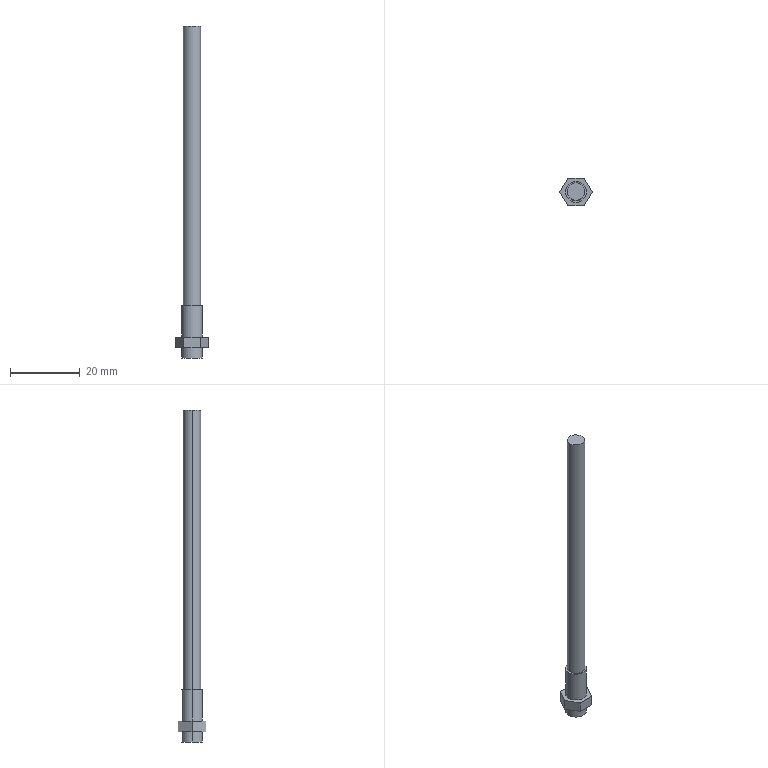Part | SolidWorks | features BaseBody 1 | 1 solid | 17 faces | box 9.238 x 8 x 95 mm | volume 2076 mm3 | plane 11 | cylinder 6 | commonest cylinder face diameters 6 x4 5 x2
STEP:
#1=CARTESIAN_POINT('',(-3.,0.,-15.));
#2=VERTEX_POINT('',#1);
#3=CARTESIAN_POINT('',(3.,0.,-15.));
#4=VERTEX_POINT('',#3);
#5=CARTESIAN_POINT('',(0.,0.,-15.));
#6=DIRECTION('',(0.,0.,-1.));
#7=DIRECTION('',(-1.,0.,0.));
#8=AXIS2_PLACEMENT_3D('',#5,#6,#7);
#9=CIRCLE('',#8,3.);
#10=EDGE_CURVE('',#2,#4,#9,.T.);
#11=ORIENTED_EDGE('',*,*,#10,.F.);
#12=CARTESIAN_POINT('',(-3.,0.,-12.));
#13=VERTEX_POINT('',#12);
#14=CARTESIAN_POINT('',(-3.,0.,-15.));
#15=DIRECTION('',(0.,0.,1.));
#16=VECTOR('',#15,1000.);
#17=LINE('',#14,#16);
#18=EDGE_CURVE('',#2,#13,#17,.T.);
#19=ORIENTED_EDGE('',*,*,#18,.T.);
#20=CARTESIAN_POINT('',(3.,0.,-12.));
#21=VERTEX_POINT('',#20);
#22=CARTESIAN_POINT('',(0.,0.,-12.));
#23=DIRECTION('',(0.,0.,-1.));
#24=DIRECTION('',(-1.,0.,0.));
#25=AXIS2_PLACEMENT_3D('',#22,#23,#24);
#26=CIRCLE('',#25,3.);
#27=EDGE_CURVE('',#13,#21,#26,.T.);
#28=ORIENTED_EDGE('',*,*,#27,.T.);
#29=CARTESIAN_POINT('',(3.,0.,-15.));
#30=DIRECTION('',(0.,0.,1.));
#31=VECTOR('',#30,1000.);
#32=LINE('',#29,#31);
#33=EDGE_CURVE('',#4,#21,#32,.T.);
#34=ORIENTED_EDGE('',*,*,#33,.F.);
#35=EDGE_LOOP('',(#11,#19,#28,#34));
#36=FACE_OUTER_BOUND('',#35,.T.);
#37=CARTESIAN_POINT('',(0.,0.,-15.));
#38=DIRECTION('',(0.,0.,1.));
#39=DIRECTION('',(1.,0.,0.));
#40=AXIS2_PLACEMENT_3D('',#37,#38,#39);
#41=CYLINDRICAL_SURFACE('',#40,3.);
#42=ADVANCED_FACE('',(#36),#41,.T.);
#43=CARTESIAN_POINT('',(2.5,0.,80.));
#44=VERTEX_POINT('',#43);
#45=CARTESIAN_POINT('',(-2.5,0.,80.));
#46=VERTEX_POINT('',#45);
#47=CARTESIAN_POINT('',(0.,0.,80.));
#48=DIRECTION('',(0.,0.,1.));
#49=DIRECTION('',(1.,0.,0.));
#50=AXIS2_PLACEMENT_3D('',#47,#48,#49);
#51=CIRCLE('',#50,2.5);
#52=EDGE_CURVE('',#44,#46,#51,.T.);
#53=ORIENTED_EDGE('',*,*,#52,.F.);
#54=CARTESIAN_POINT('',(2.5,0.,0.));
#55=VERTEX_POINT('',#54);
#56=CARTESIAN_POINT('',(2.5,0.,80.));
#57=DIRECTION('',(0.,0.,-1.));
#58=VECTOR('',#57,1000.);
#59=LINE('',#56,#58);
#60=EDGE_CURVE('',#44,#55,#59,.T.);
#61=ORIENTED_EDGE('',*,*,#60,.T.);
#62=CARTESIAN_POINT('',(-2.5,0.,0.));
#63=VERTEX_POINT('',#62);
#64=CARTESIAN_POINT('',(0.,0.,0.));
#65=DIRECTION('',(0.,0.,1.));
#66=DIRECTION('',(1.,0.,0.));
#67=AXIS2_PLACEMENT_3D('',#64,#65,#66);
#68=CIRCLE('',#67,2.5);
#69=EDGE_CURVE('',#55,#63,#68,.T.);
#70=ORIENTED_EDGE('',*,*,#69,.T.);
#71=CARTESIAN_POINT('',(-2.5,0.,80.));
#72=DIRECTION('',(0.,0.,-1.));
#73=VECTOR('',#72,1000.);
#74=LINE('',#71,#73);
#75=EDGE_CURVE('',#46,#63,#74,.T.);
#76=ORIENTED_EDGE('',*,*,#75,.F.);
#77=EDGE_LOOP('',(#53,#61,#70,#76));
#78=FACE_OUTER_BOUND('',#77,.T.);
#79=CARTESIAN_POINT('',(0.,0.,80.));
#80=DIRECTION('',(0.,0.,-1.));
#81=DIRECTION('',(-1.,0.,0.));
#82=AXIS2_PLACEMENT_3D('',#79,#80,#81);
#83=CYLINDRICAL_SURFACE('',#82,2.5);
#84=ADVANCED_FACE('',(#78),#83,.T.);
#85=CARTESIAN_POINT('',(-3.,0.,-9.));
#86=VERTEX_POINT('',#85);
#87=CARTESIAN_POINT('',(3.,0.,-9.));
#88=VERTEX_POINT('',#87);
#89=CARTESIAN_POINT('',(0.,0.,-9.));
#90=DIRECTION('',(0.,0.,-1.));
#91=DIRECTION('',(-1.,0.,0.));
#92=AXIS2_PLACEMENT_3D('',#89,#90,#91);
#93=CIRCLE('',#92,3.);
#94=EDGE_CURVE('',#86,#88,#93,.T.);
#95=ORIENTED_EDGE('',*,*,#94,.F.);
#96=CARTESIAN_POINT('',(-3.,0.,0.));
#97=VERTEX_POINT('',#96);
#98=CARTESIAN_POINT('',(-3.,0.,-15.));
#99=DIRECTION('',(0.,0.,1.));
#100=VECTOR('',#99,1000.);
#101=LINE('',#98,#100);
#102=EDGE_CURVE('',#86,#97,#101,.T.);
#103=ORIENTED_EDGE('',*,*,#102,.T.);
#104=CARTESIAN_POINT('',(3.,0.,0.));
#105=VERTEX_POINT('',#104);
#106=CARTESIAN_POINT('',(0.,0.,0.));
#107=DIRECTION('',(0.,0.,-1.));
#108=DIRECTION('',(-1.,0.,0.));
#109=AXIS2_PLACEMENT_3D('',#106,#107,#108);
#110=CIRCLE('',#109,3.);
#111=EDGE_CURVE('',#97,#105,#110,.T.);
#112=ORIENTED_EDGE('',*,*,#111,.T.);
#113=CARTESIAN_POINT('',(3.,0.,-15.));
#114=DIRECTION('',(0.,0.,1.));
#115=VECTOR('',#114,1000.);
#116=LINE('',#113,#115);
#117=EDGE_CURVE('',#88,#105,#116,.T.);
#118=ORIENTED_EDGE('',*,*,#117,.F.);
#119=EDGE_LOOP('',(#95,#103,#112,#118));
#120=FACE_OUTER_BOUND('',#119,.T.);
#121=CARTESIAN_POINT('',(0.,0.,-15.));
#122=DIRECTION('',(0.,0.,1.));
#123=DIRECTION('',(1.,0.,0.));
#124=AXIS2_PLACEMENT_3D('',#121,#122,#123);
#125=CYLINDRICAL_SURFACE('',#124,3.);
#126=ADVANCED_FACE('',(#120),#125,.T.);
#127=CARTESIAN_POINT('',(0.,0.,-15.));
#128=DIRECTION('',(0.,0.,-1.));
#129=DIRECTION('',(-1.,0.,0.));
#130=AXIS2_PLACEMENT_3D('',#127,#128,#129);
#131=CIRCLE('',#130,3.);
#132=EDGE_CURVE('',#4,#2,#131,.T.);
#133=ORIENTED_EDGE('',*,*,#132,.T.);
#134=ORIENTED_EDGE('',*,*,#10,.T.);
#135=EDGE_LOOP('',(#133,#134));
#136=FACE_OUTER_BOUND('',#135,.T.);
#137=CARTESIAN_POINT('',(0.,0.,-15.));
#138=DIRECTION('',(0.,0.,-1.));
#139=DIRECTION('',(0.,-1.,0.));
#140=AXIS2_PLACEMENT_3D('',#137,#138,#139);
#141=PLANE('',#140);
#142=ADVANCED_FACE('',(#136),#141,.T.);
#143=CARTESIAN_POINT('',(0.,0.,-9.));
#144=DIRECTION('',(0.,0.,-1.));
#145=DIRECTION('',(-1.,0.,0.));
#146=AXIS2_PLACEMENT_3D('',#143,#144,#145);
#147=CIRCLE('',#146,3.);
#148=EDGE_CURVE('',#88,#86,#147,.T.);
#149=ORIENTED_EDGE('',*,*,#148,.T.);
#150=ORIENTED_EDGE('',*,*,#94,.T.);
#151=EDGE_LOOP('',(#149,#150));
#152=FACE_BOUND('',#151,.T.);
#153=CARTESIAN_POINT('',(-2.309,-4.,-9.));
#154=VERTEX_POINT('',#153);
#155=CARTESIAN_POINT('',(-4.619,0.,-9.));
#156=VERTEX_POINT('',#155);
#157=CARTESIAN_POINT('',(-2.309,-4.,-9.));
#158=DIRECTION('',(-0.5,0.866,0.));
#159=VECTOR('',#158,1000.);
#160=LINE('',#157,#159);
#161=EDGE_CURVE('',#154,#156,#160,.T.);
#162=ORIENTED_EDGE('',*,*,#161,.F.);
#163=CARTESIAN_POINT('',(2.309,-4.,-9.));
#164=VERTEX_POINT('',#163);
#165=CARTESIAN_POINT('',(2.309,-4.,-9.));
#166=DIRECTION('',(-1.,0.,0.));
#167=VECTOR('',#166,1000.);
#168=LINE('',#165,#167);
#169=EDGE_CURVE('',#164,#154,#168,.T.);
#170=ORIENTED_EDGE('',*,*,#169,.F.);
#171=CARTESIAN_POINT('',(4.619,0.,-9.));
#172=VERTEX_POINT('',#171);
#173=CARTESIAN_POINT('',(4.619,0.,-9.));
#174=DIRECTION('',(-0.5,-0.866,0.));
#175=VECTOR('',#174,1000.);
#176=LINE('',#173,#175);
#177=EDGE_CURVE('',#172,#164,#176,.T.);
#178=ORIENTED_EDGE('',*,*,#177,.F.);
#179=CARTESIAN_POINT('',(2.309,4.,-9.));
#180=VERTEX_POINT('',#179);
#181=CARTESIAN_POINT('',(2.309,4.,-9.));
#182=DIRECTION('',(0.5,-0.866,0.));
#183=VECTOR('',#182,1000.);
#184=LINE('',#181,#183);
#185=EDGE_CURVE('',#180,#172,#184,.T.);
#186=ORIENTED_EDGE('',*,*,#185,.F.);
#187=CARTESIAN_POINT('',(-2.309,4.,-9.));
#188=VERTEX_POINT('',#187);
#189=CARTESIAN_POINT('',(-2.309,4.,-9.));
#190=DIRECTION('',(1.,0.,0.));
#191=VECTOR('',#190,1000.);
#192=LINE('',#189,#191);
#193=EDGE_CURVE('',#188,#180,#192,.T.);
#194=ORIENTED_EDGE('',*,*,#193,.F.);
#195=CARTESIAN_POINT('',(-4.619,0.,-9.));
#196=DIRECTION('',(0.5,0.866,0.));
#197=VECTOR('',#196,1000.);
#198=LINE('',#195,#197);
#199=EDGE_CURVE('',#156,#188,#198,.T.);
#200=ORIENTED_EDGE('',*,*,#199,.F.);
#201=EDGE_LOOP('',(#162,#170,#178,#186,#194,#200));
#202=FACE_OUTER_BOUND('',#201,.T.);
#203=CARTESIAN_POINT('',(0.,0.,-9.));
#204=DIRECTION('',(0.,0.,-1.));
#205=DIRECTION('',(0.,-1.,0.));
#206=AXIS2_PLACEMENT_3D('',#203,#204,#205);
#207=PLANE('',#206);
#208=ADVANCED_FACE('',(#152,#202),#207,.F.);
#209=CARTESIAN_POINT('',(0.,0.,-12.));
#210=DIRECTION('',(0.,0.,-1.));
#211=DIRECTION('',(-1.,0.,0.));
#212=AXIS2_PLACEMENT_3D('',#209,#210,#211);
#213=CIRCLE('',#212,3.);
#214=EDGE_CURVE('',#21,#13,#213,.T.);
#215=ORIENTED_EDGE('',*,*,#214,.F.);
#216=ORIENTED_EDGE('',*,*,#27,.F.);
#217=EDGE_LOOP('',(#215,#216));
#218=FACE_BOUND('',#217,.T.);
#219=CARTESIAN_POINT('',(-2.309,-4.,-12.));
#220=VERTEX_POINT('',#219);
#221=CARTESIAN_POINT('',(-4.619,0.,-12.));
#222=VERTEX_POINT('',#221);
#223=CARTESIAN_POINT('',(-2.309,-4.,-12.));
#224=DIRECTION('',(-0.5,0.866,0.));
#225=VECTOR('',#224,1000.);
#226=LINE('',#223,#225);
#227=EDGE_CURVE('',#220,#222,#226,.T.);
#228=ORIENTED_EDGE('',*,*,#227,.T.);
#229=CARTESIAN_POINT('',(-2.309,4.,-12.));
#230=VERTEX_POINT('',#229);
#231=CARTESIAN_POINT('',(-4.619,0.,-12.));
#232=DIRECTION('',(0.5,0.866,0.));
#233=VECTOR('',#232,1000.);
#234=LINE('',#231,#233);
#235=EDGE_CURVE('',#222,#230,#234,.T.);
#236=ORIENTED_EDGE('',*,*,#235,.T.);
#237=CARTESIAN_POINT('',(2.309,4.,-12.));
#238=VERTEX_POINT('',#237);
#239=CARTESIAN_POINT('',(-2.309,4.,-12.));
#240=DIRECTION('',(1.,0.,0.));
#241=VECTOR('',#240,1000.);
#242=LINE('',#239,#241);
#243=EDGE_CURVE('',#230,#238,#242,.T.);
#244=ORIENTED_EDGE('',*,*,#243,.T.);
#245=CARTESIAN_POINT('',(4.619,0.,-12.));
#246=VERTEX_POINT('',#245);
#247=CARTESIAN_POINT('',(2.309,4.,-12.));
#248=DIRECTION('',(0.5,-0.866,0.));
#249=VECTOR('',#248,1000.);
#250=LINE('',#247,#249);
#251=EDGE_CURVE('',#238,#246,#250,.T.);
#252=ORIENTED_EDGE('',*,*,#251,.T.);
#253=CARTESIAN_POINT('',(2.309,-4.,-12.));
#254=VERTEX_POINT('',#253);
#255=CARTESIAN_POINT('',(4.619,0.,-12.));
#256=DIRECTION('',(-0.5,-0.866,0.));
#257=VECTOR('',#256,1000.);
#258=LINE('',#255,#257);
#259=EDGE_CURVE('',#246,#254,#258,.T.);
#260=ORIENTED_EDGE('',*,*,#259,.T.);
#261=CARTESIAN_POINT('',(2.309,-4.,-12.));
#262=DIRECTION('',(-1.,0.,0.));
#263=VECTOR('',#262,1000.);
#264=LINE('',#261,#263);
#265=EDGE_CURVE('',#254,#220,#264,.T.);
#266=ORIENTED_EDGE('',*,*,#265,.T.);
#267=EDGE_LOOP('',(#228,#236,#244,#252,#260,#266));
#268=FACE_OUTER_BOUND('',#267,.T.);
#269=CARTESIAN_POINT('',(0.,0.,-12.));
#270=DIRECTION('',(0.,0.,-1.));
#271=DIRECTION('',(0.,-1.,0.));
#272=AXIS2_PLACEMENT_3D('',#269,#270,#271);
#273=PLANE('',#272);
#274=ADVANCED_FACE('',(#218,#268),#273,.T.);
#275=ORIENTED_EDGE('',*,*,#169,.T.);
#276=CARTESIAN_POINT('',(-2.309,-4.,-12.));
#277=DIRECTION('',(0.,0.,1.));
#278=VECTOR('',#277,1000.);
#279=LINE('',#276,#278);
#280=EDGE_CURVE('',#220,#154,#279,.T.);
#281=ORIENTED_EDGE('',*,*,#280,.F.);
#282=ORIENTED_EDGE('',*,*,#265,.F.);
#283=CARTESIAN_POINT('',(2.309,-4.,-12.));
#284=DIRECTION('',(0.,0.,1.));
#285=VECTOR('',#284,1000.);
#286=LINE('',#283,#285);
#287=EDGE_CURVE('',#254,#164,#286,.T.);
#288=ORIENTED_EDGE('',*,*,#287,.T.);
#289=EDGE_LOOP('',(#275,#281,#282,#288));
#290=FACE_OUTER_BOUND('',#289,.T.);
#291=CARTESIAN_POINT('',(2.309,-4.,-12.));
#292=DIRECTION('',(0.,1.,0.));
#293=DIRECTION('',(1.,0.,0.));
#294=AXIS2_PLACEMENT_3D('',#291,#292,#293);
#295=PLANE('',#294);
#296=ADVANCED_FACE('',(#290),#295,.F.);
#297=ORIENTED_EDGE('',*,*,#177,.T.);
#298=ORIENTED_EDGE('',*,*,#287,.F.);
#299=ORIENTED_EDGE('',*,*,#259,.F.);
#300=CARTESIAN_POINT('',(4.619,0.,-12.));
#301=DIRECTION('',(0.,0.,1.));
#302=VECTOR('',#301,1000.);
#303=LINE('',#300,#302);
#304=EDGE_CURVE('',#246,#172,#303,.T.);
#305=ORIENTED_EDGE('',*,*,#304,.T.);
#306=EDGE_LOOP('',(#297,#298,#299,#305));
#307=FACE_OUTER_BOUND('',#306,.T.);
#308=CARTESIAN_POINT('',(4.619,0.,-12.));
#309=DIRECTION('',(-0.866,0.5,0.));
#310=DIRECTION('',(0.,0.,1.));
#311=AXIS2_PLACEMENT_3D('',#308,#309,#310);
#312=PLANE('',#311);
#313=ADVANCED_FACE('',(#307),#312,.F.);
#314=ORIENTED_EDGE('',*,*,#185,.T.);
#315=ORIENTED_EDGE('',*,*,#304,.F.);
#316=ORIENTED_EDGE('',*,*,#251,.F.);
#317=CARTESIAN_POINT('',(2.309,4.,-12.));
#318=DIRECTION('',(0.,0.,1.));
#319=VECTOR('',#318,1000.);
#320=LINE('',#317,#319);
#321=EDGE_CURVE('',#238,#180,#320,.T.);
#322=ORIENTED_EDGE('',*,*,#321,.T.);
#323=EDGE_LOOP('',(#314,#315,#316,#322));
#324=FACE_OUTER_BOUND('',#323,.T.);
#325=CARTESIAN_POINT('',(2.309,4.,-12.));
#326=DIRECTION('',(-0.866,-0.5,0.));
#327=DIRECTION('',(-0.5,0.866,0.));
#328=AXIS2_PLACEMENT_3D('',#325,#326,#327);
#329=PLANE('',#328);
#330=ADVANCED_FACE('',(#324),#329,.F.);
#331=ORIENTED_EDGE('',*,*,#193,.T.);
#332=ORIENTED_EDGE('',*,*,#321,.F.);
#333=ORIENTED_EDGE('',*,*,#243,.F.);
#334=CARTESIAN_POINT('',(-2.309,4.,-12.));
#335=DIRECTION('',(0.,0.,1.));
#336=VECTOR('',#335,1000.);
#337=LINE('',#334,#336);
#338=EDGE_CURVE('',#230,#188,#337,.T.);
#339=ORIENTED_EDGE('',*,*,#338,.T.);
#340=EDGE_LOOP('',(#331,#332,#333,#339));
#341=FACE_OUTER_BOUND('',#340,.T.);
#342=CARTESIAN_POINT('',(-2.309,4.,-12.));
#343=DIRECTION('',(0.,-1.,0.));
#344=DIRECTION('',(-1.,0.,0.));
#345=AXIS2_PLACEMENT_3D('',#342,#343,#344);
#346=PLANE('',#345);
#347=ADVANCED_FACE('',(#341),#346,.F.);
#348=ORIENTED_EDGE('',*,*,#199,.T.);
#349=ORIENTED_EDGE('',*,*,#338,.F.);
#350=ORIENTED_EDGE('',*,*,#235,.F.);
#351=CARTESIAN_POINT('',(-4.619,0.,-12.));
#352=DIRECTION('',(0.,0.,1.));
#353=VECTOR('',#352,1000.);
#354=LINE('',#351,#353);
#355=EDGE_CURVE('',#222,#156,#354,.T.);
#356=ORIENTED_EDGE('',*,*,#355,.T.);
#357=EDGE_LOOP('',(#348,#349,#350,#356));
#358=FACE_OUTER_BOUND('',#357,.T.);
#359=CARTESIAN_POINT('',(-4.619,0.,-12.));
#360=DIRECTION('',(0.866,-0.5,0.));
#361=DIRECTION('',(0.,0.,-1.));
#362=AXIS2_PLACEMENT_3D('',#359,#360,#361);
#363=PLANE('',#362);
#364=ADVANCED_FACE('',(#358),#363,.F.);
#365=ORIENTED_EDGE('',*,*,#161,.T.);
#366=ORIENTED_EDGE('',*,*,#355,.F.);
#367=ORIENTED_EDGE('',*,*,#227,.F.);
#368=ORIENTED_EDGE('',*,*,#280,.T.);
#369=EDGE_LOOP('',(#365,#366,#367,#368));
#370=FACE_OUTER_BOUND('',#369,.T.);
#371=CARTESIAN_POINT('',(-2.309,-4.,-12.));
#372=DIRECTION('',(0.866,0.5,0.));
#373=DIRECTION('',(0.,0.,-1.));
#374=AXIS2_PLACEMENT_3D('',#371,#372,#373);
#375=PLANE('',#374);
#376=ADVANCED_FACE('',(#370),#375,.F.);
#377=CARTESIAN_POINT('',(0.,0.,0.));
#378=DIRECTION('',(0.,0.,1.));
#379=DIRECTION('',(1.,0.,0.));
#380=AXIS2_PLACEMENT_3D('',#377,#378,#379);
#381=CIRCLE('',#380,2.5);
#382=EDGE_CURVE('',#63,#55,#381,.T.);
#383=ORIENTED_EDGE('',*,*,#382,.F.);
#384=ORIENTED_EDGE('',*,*,#69,.F.);
#385=EDGE_LOOP('',(#383,#384));
#386=FACE_BOUND('',#385,.T.);
#387=CARTESIAN_POINT('',(0.,0.,0.));
#388=DIRECTION('',(0.,0.,-1.));
#389=DIRECTION('',(-1.,0.,0.));
#390=AXIS2_PLACEMENT_3D('',#387,#388,#389);
#391=CIRCLE('',#390,3.);
#392=EDGE_CURVE('',#105,#97,#391,.T.);
#393=ORIENTED_EDGE('',*,*,#392,.F.);
#394=ORIENTED_EDGE('',*,*,#111,.F.);
#395=EDGE_LOOP('',(#393,#394));
#396=FACE_OUTER_BOUND('',#395,.T.);
#397=CARTESIAN_POINT('',(0.,0.,0.));
#398=DIRECTION('',(0.,0.,-1.));
#399=DIRECTION('',(0.,-1.,0.));
#400=AXIS2_PLACEMENT_3D('',#397,#398,#399);
#401=PLANE('',#400);
#402=ADVANCED_FACE('',(#386,#396),#401,.F.);
#403=CARTESIAN_POINT('',(0.,0.,80.));
#404=DIRECTION('',(0.,0.,1.));
#405=DIRECTION('',(1.,0.,0.));
#406=AXIS2_PLACEMENT_3D('',#403,#404,#405);
#407=CIRCLE('',#406,2.5);
#408=EDGE_CURVE('',#46,#44,#407,.T.);
#409=ORIENTED_EDGE('',*,*,#408,.T.);
#410=ORIENTED_EDGE('',*,*,#52,.T.);
#411=EDGE_LOOP('',(#409,#410));
#412=FACE_OUTER_BOUND('',#411,.T.);
#413=CARTESIAN_POINT('',(0.,0.,80.));
#414=DIRECTION('',(0.,0.,1.));
#415=DIRECTION('',(1.,0.,0.));
#416=AXIS2_PLACEMENT_3D('',#413,#414,#415);
#417=PLANE('',#416);
#418=ADVANCED_FACE('',(#412),#417,.T.);
#419=ORIENTED_EDGE('',*,*,#102,.F.);
#420=ORIENTED_EDGE('',*,*,#148,.F.);
#421=ORIENTED_EDGE('',*,*,#117,.T.);
#422=ORIENTED_EDGE('',*,*,#392,.T.);
#423=EDGE_LOOP('',(#419,#420,#421,#422));
#424=FACE_OUTER_BOUND('',#423,.T.);
#425=CARTESIAN_POINT('',(0.,0.,-15.));
#426=DIRECTION('',(0.,0.,1.));
#427=DIRECTION('',(1.,0.,0.));
#428=AXIS2_PLACEMENT_3D('',#425,#426,#427);
#429=CYLINDRICAL_SURFACE('',#428,3.);
#430=ADVANCED_FACE('',(#424),#429,.T.);
#431=ORIENTED_EDGE('',*,*,#60,.F.);
#432=ORIENTED_EDGE('',*,*,#408,.F.);
#433=ORIENTED_EDGE('',*,*,#75,.T.);
#434=ORIENTED_EDGE('',*,*,#382,.T.);
#435=EDGE_LOOP('',(#431,#432,#433,#434));
#436=FACE_OUTER_BOUND('',#435,.T.);
#437=CARTESIAN_POINT('',(0.,0.,80.));
#438=DIRECTION('',(0.,0.,-1.));
#439=DIRECTION('',(-1.,0.,0.));
#440=AXIS2_PLACEMENT_3D('',#437,#438,#439);
#441=CYLINDRICAL_SURFACE('',#440,2.5);
#442=ADVANCED_FACE('',(#436),#441,.T.);
#443=ORIENTED_EDGE('',*,*,#18,.F.);
#444=ORIENTED_EDGE('',*,*,#132,.F.);
#445=ORIENTED_EDGE('',*,*,#33,.T.);
#446=ORIENTED_EDGE('',*,*,#214,.T.);
#447=EDGE_LOOP('',(#443,#444,#445,#446));
#448=FACE_OUTER_BOUND('',#447,.T.);
#449=CARTESIAN_POINT('',(0.,0.,-15.));
#450=DIRECTION('',(0.,0.,1.));
#451=DIRECTION('',(1.,0.,0.));
#452=AXIS2_PLACEMENT_3D('',#449,#450,#451);
#453=CYLINDRICAL_SURFACE('',#452,3.);
#454=ADVANCED_FACE('',(#448),#453,.T.);
#455=CLOSED_SHELL('',(#42,#84,#126,#142,#208,#274,#296,#313,#330,#347,#364,#376,#402,#418,#430,#442,#454));
#456=MANIFOLD_SOLID_BREP('',#455);
#457=CARTESIAN_POINT('',(0.,0.,0.));
#458=DIRECTION('',(0.,0.,1.));
#459=DIRECTION('',(1.,0.,0.));
#460=AXIS2_PLACEMENT_3D('',#457,#458,#459);
#461=(LENGTH_UNIT()NAMED_UNIT(*)SI_UNIT(.MILLI.,.METRE.));
#462=UNCERTAINTY_MEASURE_WITH_UNIT(LENGTH_MEASURE(0.00001),#461,'','');
#463=(NAMED_UNIT(*)PLANE_ANGLE_UNIT()SI_UNIT($,.RADIAN.));
#464=(NAMED_UNIT(*)SI_UNIT($,.STERADIAN.)SOLID_ANGLE_UNIT());
#465=(GEOMETRIC_REPRESENTATION_CONTEXT(3)GLOBAL_UNCERTAINTY_ASSIGNED_CONTEXT((#462))GLOBAL_UNIT_ASSIGNED_CONTEXT((#461,#463,#464))REPRESENTATION_CONTEXT('',''));
#466=ADVANCED_BREP_SHAPE_REPRESENTATION('',(#456,#460),#465);